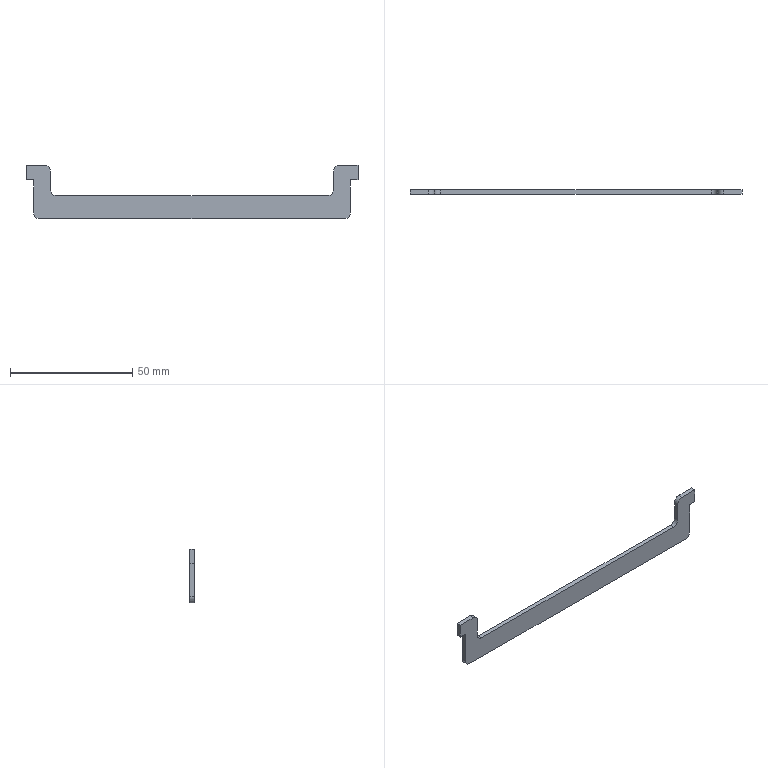Part | STEP file | 1 solid | 20 faces | box 136 x 1.85 x 22 mm | volume 2666 mm3 | plane 14 | cylinder 6 | commonest cylinder face diameters 5 x6